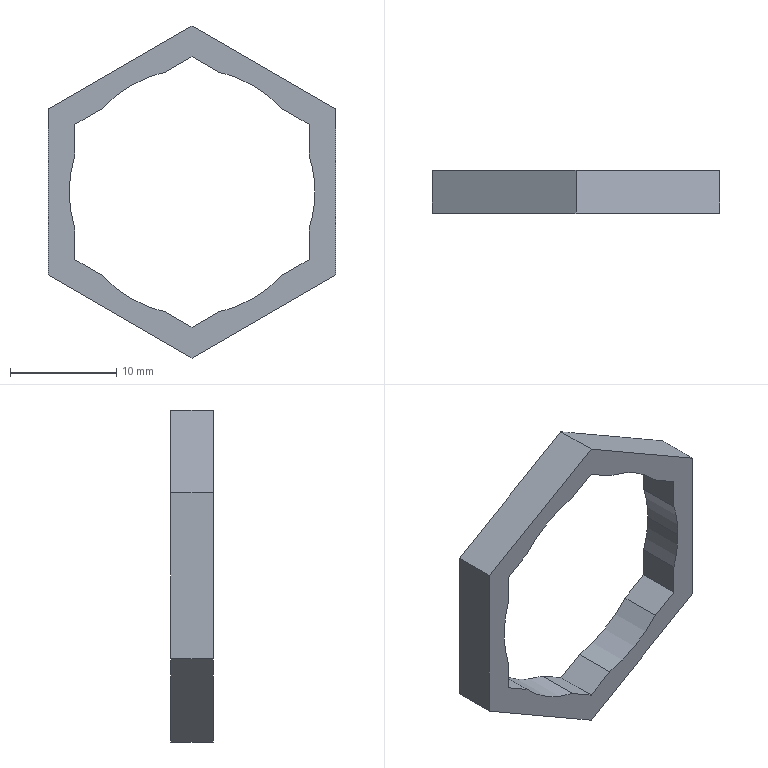Part | STEP file | Nut MS887-3-4 | 1 solid | 27 faces | box 27 x 4 x 31.177 mm | volume 789.045 mm3 | plane 20 | cylinder 7 | commonest cylinder face diameters 23.069 x7